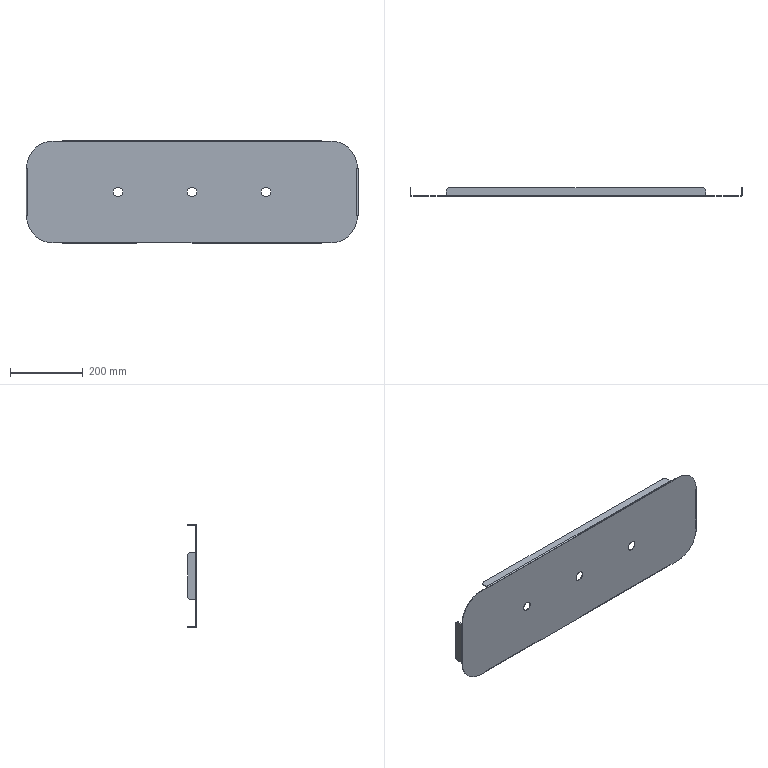Part | NX | features BREP 1 | 1 solid | 96 faces | box 911.047 x 24.105 x 282.397 mm | volume 423760 mm3 | plane 66 | cylinder 30 | commonest cylinder face diameters 19.05 x10 25.4 x6 3.175 x5 6.172 x5 146.05 x4